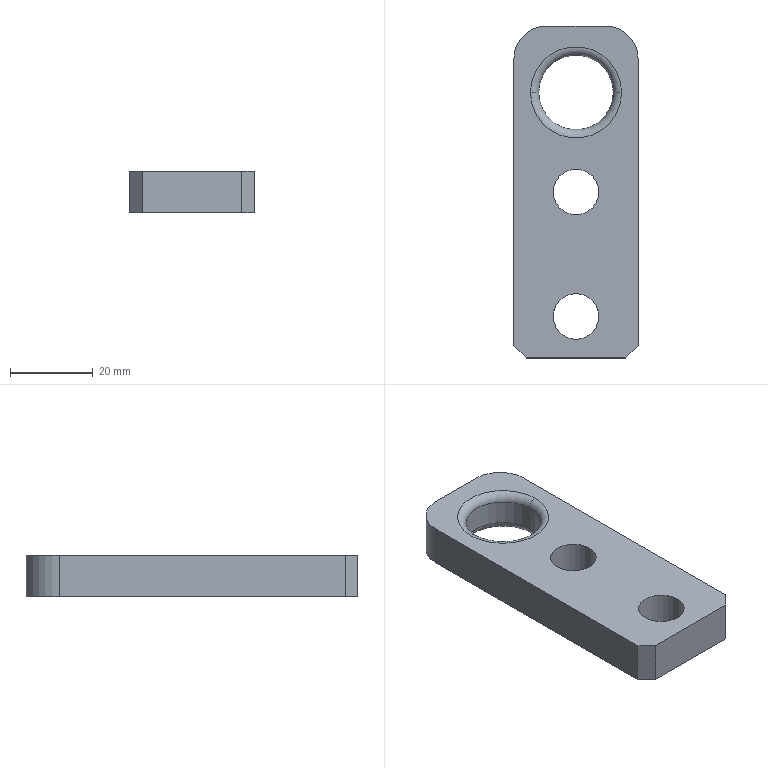Part | Creo | features DATUM PLANE 3, CHAMFER 1, COORDINATE SYSTEM 1, CURVE 1, PROTRUSION 1, ROUND 1 | 1 solid | 20 faces | box 30 x 80 x 10 mm | volume 19088 mm3 | plane 8 | cylinder 8 | torus 4 | commonest cylinder face diameters 11 x4 16 x2 18 x2
STEP:
#1=CARTESIAN_POINT('',(0.,0.,0.));
#2=DIRECTION('',(0.,0.,1.));
#3=DIRECTION('',(1.,0.,0.));
#4=AXIS2_PLACEMENT_3D('',#1,#2,#3);
#5=CARTESIAN_POINT('',(15.,-37.,0.));
#6=VERTEX_POINT('',#5);
#7=CARTESIAN_POINT('',(12.,-40.,0.));
#8=VERTEX_POINT('',#7);
#9=CARTESIAN_POINT('',(15.,-37.,0.));
#10=DIRECTION('',(-0.7071,-0.7071,0.));
#11=VECTOR('',#10,4.243);
#12=LINE('',#9,#11);
#13=EDGE_CURVE('',#6,#8,#12,.T.);
#14=ORIENTED_EDGE('',*,*,#13,.F.);
#15=CARTESIAN_POINT('',(15.,32.,0.));
#16=VERTEX_POINT('',#15);
#17=CARTESIAN_POINT('',(15.,-37.,0.));
#18=DIRECTION('',(0.,1.,0.));
#19=VECTOR('',#18,69.);
#20=LINE('',#17,#19);
#21=EDGE_CURVE('',#6,#16,#20,.T.);
#22=ORIENTED_EDGE('',*,*,#21,.T.);
#23=CARTESIAN_POINT('',(7.,40.,0.));
#24=VERTEX_POINT('',#23);
#25=CARTESIAN_POINT('',(7.,32.,0.));
#26=DIRECTION('',(0.,0.,1.));
#27=DIRECTION('',(1.,0.,0.));
#28=AXIS2_PLACEMENT_3D('',#25,#26,#27);
#29=CIRCLE('',#28,8.);
#30=EDGE_CURVE('',#16,#24,#29,.T.);
#31=ORIENTED_EDGE('',*,*,#30,.T.);
#32=CARTESIAN_POINT('',(-7.,40.,0.));
#33=VERTEX_POINT('',#32);
#34=CARTESIAN_POINT('',(7.,40.,0.));
#35=DIRECTION('',(-1.,0.,0.));
#36=VECTOR('',#35,14.);
#37=LINE('',#34,#36);
#38=EDGE_CURVE('',#24,#33,#37,.T.);
#39=ORIENTED_EDGE('',*,*,#38,.T.);
#40=CARTESIAN_POINT('',(-15.,32.,0.));
#41=VERTEX_POINT('',#40);
#42=CARTESIAN_POINT('',(-7.,32.,0.));
#43=DIRECTION('',(0.,0.,1.));
#44=DIRECTION('',(0.,1.,0.));
#45=AXIS2_PLACEMENT_3D('',#42,#43,#44);
#46=CIRCLE('',#45,8.);
#47=EDGE_CURVE('',#33,#41,#46,.T.);
#48=ORIENTED_EDGE('',*,*,#47,.T.);
#49=CARTESIAN_POINT('',(-15.,-37.,0.));
#50=VERTEX_POINT('',#49);
#51=CARTESIAN_POINT('',(-15.,32.,0.));
#52=DIRECTION('',(0.,-1.,0.));
#53=VECTOR('',#52,69.);
#54=LINE('',#51,#53);
#55=EDGE_CURVE('',#41,#50,#54,.T.);
#56=ORIENTED_EDGE('',*,*,#55,.T.);
#57=CARTESIAN_POINT('',(-12.,-40.,0.));
#58=VERTEX_POINT('',#57);
#59=CARTESIAN_POINT('',(-12.,-40.,0.));
#60=DIRECTION('',(-0.7071,0.7071,0.));
#61=VECTOR('',#60,4.243);
#62=LINE('',#59,#61);
#63=EDGE_CURVE('',#58,#50,#62,.T.);
#64=ORIENTED_EDGE('',*,*,#63,.F.);
#65=CARTESIAN_POINT('',(-12.,-40.,0.));
#66=DIRECTION('',(1.,0.,0.));
#67=VECTOR('',#66,24.);
#68=LINE('',#65,#67);
#69=EDGE_CURVE('',#58,#8,#68,.T.);
#70=ORIENTED_EDGE('',*,*,#69,.T.);
#71=EDGE_LOOP('',(#14,#22,#31,#39,#48,#56,#64,#70));
#72=FACE_OUTER_BOUND('',#71,.F.);
#73=CARTESIAN_POINT('',(5.5,0.,0.));
#74=VERTEX_POINT('',#73);
#75=CARTESIAN_POINT('',(-5.5,0.,0.));
#76=VERTEX_POINT('',#75);
#77=CARTESIAN_POINT('',(0.,0.,0.));
#78=DIRECTION('',(0.,0.,-1.));
#79=DIRECTION('',(1.,0.,0.));
#80=AXIS2_PLACEMENT_3D('',#77,#78,#79);
#81=CIRCLE('',#80,5.5);
#82=EDGE_CURVE('',#74,#76,#81,.T.);
#83=ORIENTED_EDGE('',*,*,#82,.T.);
#84=CARTESIAN_POINT('',(0.,0.,0.));
#85=DIRECTION('',(0.,0.,-1.));
#86=DIRECTION('',(-1.,0.,0.));
#87=AXIS2_PLACEMENT_3D('',#84,#85,#86);
#88=CIRCLE('',#87,5.5);
#89=EDGE_CURVE('',#76,#74,#88,.T.);
#90=ORIENTED_EDGE('',*,*,#89,.T.);
#91=EDGE_LOOP('',(#83,#90));
#92=FACE_BOUND('',#91,.F.);
#93=CARTESIAN_POINT('',(5.5,-30.,0.));
#94=VERTEX_POINT('',#93);
#95=CARTESIAN_POINT('',(-5.5,-30.,0.));
#96=VERTEX_POINT('',#95);
#97=CARTESIAN_POINT('',(0.,-30.,0.));
#98=DIRECTION('',(0.,0.,-1.));
#99=DIRECTION('',(1.,0.,0.));
#100=AXIS2_PLACEMENT_3D('',#97,#98,#99);
#101=CIRCLE('',#100,5.5);
#102=EDGE_CURVE('',#94,#96,#101,.T.);
#103=ORIENTED_EDGE('',*,*,#102,.T.);
#104=CARTESIAN_POINT('',(0.,-30.,0.));
#105=DIRECTION('',(0.,0.,-1.));
#106=DIRECTION('',(-1.,0.,0.));
#107=AXIS2_PLACEMENT_3D('',#104,#105,#106);
#108=CIRCLE('',#107,5.5);
#109=EDGE_CURVE('',#96,#94,#108,.T.);
#110=ORIENTED_EDGE('',*,*,#109,.T.);
#111=EDGE_LOOP('',(#103,#110));
#112=FACE_BOUND('',#111,.F.);
#113=CARTESIAN_POINT('',(-11.,24.,0.));
#114=VERTEX_POINT('',#113);
#115=CARTESIAN_POINT('',(11.,24.,0.));
#116=VERTEX_POINT('',#115);
#117=CARTESIAN_POINT('',(0.,24.,0.));
#118=DIRECTION('',(0.,0.,1.));
#119=DIRECTION('',(-1.,0.,0.));
#120=AXIS2_PLACEMENT_3D('',#117,#118,#119);
#121=CIRCLE('',#120,11.);
#122=EDGE_CURVE('',#114,#116,#121,.T.);
#123=ORIENTED_EDGE('',*,*,#122,.F.);
#124=CARTESIAN_POINT('',(0.,24.,0.));
#125=DIRECTION('',(0.,0.,1.));
#126=DIRECTION('',(1.,0.,0.));
#127=AXIS2_PLACEMENT_3D('',#124,#125,#126);
#128=CIRCLE('',#127,11.);
#129=EDGE_CURVE('',#116,#114,#128,.T.);
#130=ORIENTED_EDGE('',*,*,#129,.F.);
#131=EDGE_LOOP('',(#123,#130));
#132=FACE_BOUND('',#131,.F.);
#133=CARTESIAN_POINT('',(0.,0.,0.));
#134=DIRECTION('',(0.,0.,1.));
#135=DIRECTION('',(1.,0.,0.));
#136=AXIS2_PLACEMENT_3D('',#133,#134,#135);
#137=PLANE('',#136);
#138=ADVANCED_FACE('',(#72,#92,#112,#132),#137,.F.);
#139=ORIENTED_EDGE('',*,*,#102,.F.);
#140=CARTESIAN_POINT('',(5.5,-30.,10.));
#141=VERTEX_POINT('',#140);
#142=CARTESIAN_POINT('',(5.5,-30.,0.));
#143=DIRECTION('',(0.,0.,1.));
#144=VECTOR('',#143,10.);
#145=LINE('',#142,#144);
#146=EDGE_CURVE('',#94,#141,#145,.T.);
#147=ORIENTED_EDGE('',*,*,#146,.T.);
#148=CARTESIAN_POINT('',(-5.5,-30.,10.));
#149=VERTEX_POINT('',#148);
#150=CARTESIAN_POINT('',(0.,-30.,10.));
#151=DIRECTION('',(0.,0.,-1.));
#152=DIRECTION('',(1.,0.,0.));
#153=AXIS2_PLACEMENT_3D('',#150,#151,#152);
#154=CIRCLE('',#153,5.5);
#155=EDGE_CURVE('',#141,#149,#154,.T.);
#156=ORIENTED_EDGE('',*,*,#155,.T.);
#157=CARTESIAN_POINT('',(-5.5,-30.,0.));
#158=DIRECTION('',(0.,0.,1.));
#159=VECTOR('',#158,10.);
#160=LINE('',#157,#159);
#161=EDGE_CURVE('',#96,#149,#160,.T.);
#162=ORIENTED_EDGE('',*,*,#161,.F.);
#163=EDGE_LOOP('',(#139,#147,#156,#162));
#164=FACE_OUTER_BOUND('',#163,.F.);
#165=CARTESIAN_POINT('',(0.,-30.,0.));
#166=DIRECTION('',(0.,0.,1.));
#167=DIRECTION('',(1.,0.,0.));
#168=AXIS2_PLACEMENT_3D('',#165,#166,#167);
#169=CYLINDRICAL_SURFACE('',#168,5.5);
#170=ADVANCED_FACE('',(#164),#169,.F.);
#171=ORIENTED_EDGE('',*,*,#109,.F.);
#172=ORIENTED_EDGE('',*,*,#161,.T.);
#173=CARTESIAN_POINT('',(0.,-30.,10.));
#174=DIRECTION('',(0.,0.,-1.));
#175=DIRECTION('',(-1.,0.,0.));
#176=AXIS2_PLACEMENT_3D('',#173,#174,#175);
#177=CIRCLE('',#176,5.5);
#178=EDGE_CURVE('',#149,#141,#177,.T.);
#179=ORIENTED_EDGE('',*,*,#178,.T.);
#180=ORIENTED_EDGE('',*,*,#146,.F.);
#181=EDGE_LOOP('',(#171,#172,#179,#180));
#182=FACE_OUTER_BOUND('',#181,.F.);
#183=CARTESIAN_POINT('',(0.,-30.,0.));
#184=DIRECTION('',(0.,0.,1.));
#185=DIRECTION('',(1.,0.,0.));
#186=AXIS2_PLACEMENT_3D('',#183,#184,#185);
#187=CYLINDRICAL_SURFACE('',#186,5.5);
#188=ADVANCED_FACE('',(#182),#187,.F.);
#189=CARTESIAN_POINT('',(12.,-40.,10.));
#190=VERTEX_POINT('',#189);
#191=CARTESIAN_POINT('',(15.,-37.,10.));
#192=VERTEX_POINT('',#191);
#193=CARTESIAN_POINT('',(12.,-40.,10.));
#194=DIRECTION('',(0.7071,0.7071,0.));
#195=VECTOR('',#194,4.243);
#196=LINE('',#193,#195);
#197=EDGE_CURVE('',#190,#192,#196,.T.);
#198=ORIENTED_EDGE('',*,*,#197,.F.);
#199=CARTESIAN_POINT('',(-12.,-40.,10.));
#200=VERTEX_POINT('',#199);
#201=CARTESIAN_POINT('',(-12.,-40.,10.));
#202=DIRECTION('',(1.,0.,0.));
#203=VECTOR('',#202,24.);
#204=LINE('',#201,#203);
#205=EDGE_CURVE('',#200,#190,#204,.T.);
#206=ORIENTED_EDGE('',*,*,#205,.F.);
#207=CARTESIAN_POINT('',(-15.,-37.,10.));
#208=VERTEX_POINT('',#207);
#209=CARTESIAN_POINT('',(-15.,-37.,10.));
#210=DIRECTION('',(0.7071,-0.7071,0.));
#211=VECTOR('',#210,4.243);
#212=LINE('',#209,#211);
#213=EDGE_CURVE('',#208,#200,#212,.T.);
#214=ORIENTED_EDGE('',*,*,#213,.F.);
#215=CARTESIAN_POINT('',(-15.,32.,10.));
#216=VERTEX_POINT('',#215);
#217=CARTESIAN_POINT('',(-15.,32.,10.));
#218=DIRECTION('',(0.,-1.,0.));
#219=VECTOR('',#218,69.);
#220=LINE('',#217,#219);
#221=EDGE_CURVE('',#216,#208,#220,.T.);
#222=ORIENTED_EDGE('',*,*,#221,.F.);
#223=CARTESIAN_POINT('',(-7.,40.,10.));
#224=VERTEX_POINT('',#223);
#225=CARTESIAN_POINT('',(-7.,32.,10.));
#226=DIRECTION('',(0.,0.,1.));
#227=DIRECTION('',(0.,1.,0.));
#228=AXIS2_PLACEMENT_3D('',#225,#226,#227);
#229=CIRCLE('',#228,8.);
#230=EDGE_CURVE('',#224,#216,#229,.T.);
#231=ORIENTED_EDGE('',*,*,#230,.F.);
#232=CARTESIAN_POINT('',(7.,40.,10.));
#233=VERTEX_POINT('',#232);
#234=CARTESIAN_POINT('',(7.,40.,10.));
#235=DIRECTION('',(-1.,0.,0.));
#236=VECTOR('',#235,14.);
#237=LINE('',#234,#236);
#238=EDGE_CURVE('',#233,#224,#237,.T.);
#239=ORIENTED_EDGE('',*,*,#238,.F.);
#240=CARTESIAN_POINT('',(15.,32.,10.));
#241=VERTEX_POINT('',#240);
#242=CARTESIAN_POINT('',(7.,32.,10.));
#243=DIRECTION('',(0.,0.,1.));
#244=DIRECTION('',(1.,0.,0.));
#245=AXIS2_PLACEMENT_3D('',#242,#243,#244);
#246=CIRCLE('',#245,8.);
#247=EDGE_CURVE('',#241,#233,#246,.T.);
#248=ORIENTED_EDGE('',*,*,#247,.F.);
#249=CARTESIAN_POINT('',(15.,-37.,10.));
#250=DIRECTION('',(0.,1.,0.));
#251=VECTOR('',#250,69.);
#252=LINE('',#249,#251);
#253=EDGE_CURVE('',#192,#241,#252,.T.);
#254=ORIENTED_EDGE('',*,*,#253,.F.);
#255=EDGE_LOOP('',(#198,#206,#214,#222,#231,#239,#248,#254));
#256=FACE_OUTER_BOUND('',#255,.F.);
#257=CARTESIAN_POINT('',(5.5,0.,10.));
#258=VERTEX_POINT('',#257);
#259=CARTESIAN_POINT('',(-5.5,0.,10.));
#260=VERTEX_POINT('',#259);
#261=CARTESIAN_POINT('',(0.,0.,10.));
#262=DIRECTION('',(0.,0.,-1.));
#263=DIRECTION('',(1.,0.,0.));
#264=AXIS2_PLACEMENT_3D('',#261,#262,#263);
#265=CIRCLE('',#264,5.5);
#266=EDGE_CURVE('',#258,#260,#265,.T.);
#267=ORIENTED_EDGE('',*,*,#266,.F.);
#268=CARTESIAN_POINT('',(0.,0.,10.));
#269=DIRECTION('',(0.,0.,-1.));
#270=DIRECTION('',(-1.,0.,0.));
#271=AXIS2_PLACEMENT_3D('',#268,#269,#270);
#272=CIRCLE('',#271,5.5);
#273=EDGE_CURVE('',#260,#258,#272,.T.);
#274=ORIENTED_EDGE('',*,*,#273,.F.);
#275=EDGE_LOOP('',(#267,#274));
#276=FACE_BOUND('',#275,.F.);
#277=ORIENTED_EDGE('',*,*,#155,.F.);
#278=ORIENTED_EDGE('',*,*,#178,.F.);
#279=EDGE_LOOP('',(#277,#278));
#280=FACE_BOUND('',#279,.F.);
#281=CARTESIAN_POINT('',(11.,24.,10.));
#282=VERTEX_POINT('',#281);
#283=CARTESIAN_POINT('',(-11.,24.,10.));
#284=VERTEX_POINT('',#283);
#285=CARTESIAN_POINT('',(0.,24.,10.));
#286=DIRECTION('',(0.,0.,-1.));
#287=DIRECTION('',(1.,0.,0.));
#288=AXIS2_PLACEMENT_3D('',#285,#286,#287);
#289=CIRCLE('',#288,11.);
#290=EDGE_CURVE('',#282,#284,#289,.T.);
#291=ORIENTED_EDGE('',*,*,#290,.F.);
#292=CARTESIAN_POINT('',(0.,24.,10.));
#293=DIRECTION('',(0.,0.,-1.));
#294=DIRECTION('',(-1.,0.,0.));
#295=AXIS2_PLACEMENT_3D('',#292,#293,#294);
#296=CIRCLE('',#295,11.);
#297=EDGE_CURVE('',#284,#282,#296,.T.);
#298=ORIENTED_EDGE('',*,*,#297,.F.);
#299=EDGE_LOOP('',(#291,#298));
#300=FACE_BOUND('',#299,.F.);
#301=CARTESIAN_POINT('',(0.,0.,10.));
#302=DIRECTION('',(0.,0.,1.));
#303=DIRECTION('',(1.,0.,0.));
#304=AXIS2_PLACEMENT_3D('',#301,#302,#303);
#305=PLANE('',#304);
#306=ADVANCED_FACE('',(#256,#276,#280,#300),#305,.T.);
#307=ORIENTED_EDGE('',*,*,#82,.F.);
#308=CARTESIAN_POINT('',(5.5,0.,0.));
#309=DIRECTION('',(0.,0.,1.));
#310=VECTOR('',#309,10.);
#311=LINE('',#308,#310);
#312=EDGE_CURVE('',#74,#258,#311,.T.);
#313=ORIENTED_EDGE('',*,*,#312,.T.);
#314=ORIENTED_EDGE('',*,*,#266,.T.);
#315=CARTESIAN_POINT('',(-5.5,0.,0.));
#316=DIRECTION('',(0.,0.,1.));
#317=VECTOR('',#316,10.);
#318=LINE('',#315,#317);
#319=EDGE_CURVE('',#76,#260,#318,.T.);
#320=ORIENTED_EDGE('',*,*,#319,.F.);
#321=EDGE_LOOP('',(#307,#313,#314,#320));
#322=FACE_OUTER_BOUND('',#321,.F.);
#323=CARTESIAN_POINT('',(0.,0.,0.));
#324=DIRECTION('',(0.,0.,1.));
#325=DIRECTION('',(1.,0.,0.));
#326=AXIS2_PLACEMENT_3D('',#323,#324,#325);
#327=CYLINDRICAL_SURFACE('',#326,5.5);
#328=ADVANCED_FACE('',(#322),#327,.F.);
#329=ORIENTED_EDGE('',*,*,#89,.F.);
#330=ORIENTED_EDGE('',*,*,#319,.T.);
#331=ORIENTED_EDGE('',*,*,#273,.T.);
#332=ORIENTED_EDGE('',*,*,#312,.F.);
#333=EDGE_LOOP('',(#329,#330,#331,#332));
#334=FACE_OUTER_BOUND('',#333,.F.);
#335=CARTESIAN_POINT('',(0.,0.,0.));
#336=DIRECTION('',(0.,0.,1.));
#337=DIRECTION('',(1.,0.,0.));
#338=AXIS2_PLACEMENT_3D('',#335,#336,#337);
#339=CYLINDRICAL_SURFACE('',#338,5.5);
#340=ADVANCED_FACE('',(#334),#339,.F.);
#341=ORIENTED_EDGE('',*,*,#13,.T.);
#342=CARTESIAN_POINT('',(12.,-40.,10.));
#343=DIRECTION('',(0.,0.,-1.));
#344=VECTOR('',#343,10.);
#345=LINE('',#342,#344);
#346=EDGE_CURVE('',#190,#8,#345,.T.);
#347=ORIENTED_EDGE('',*,*,#346,.F.);
#348=ORIENTED_EDGE('',*,*,#197,.T.);
#349=CARTESIAN_POINT('',(15.,-37.,10.));
#350=DIRECTION('',(0.,0.,-1.));
#351=VECTOR('',#350,10.);
#352=LINE('',#349,#351);
#353=EDGE_CURVE('',#192,#6,#352,.T.);
#354=ORIENTED_EDGE('',*,*,#353,.T.);
#355=EDGE_LOOP('',(#341,#347,#348,#354));
#356=FACE_OUTER_BOUND('',#355,.F.);
#357=CARTESIAN_POINT('',(13.5,-38.5,5.));
#358=DIRECTION('',(0.7071,-0.7071,0.));
#359=DIRECTION('',(-0.7071,-0.7071,0.));
#360=AXIS2_PLACEMENT_3D('',#357,#358,#359);
#361=PLANE('',#360);
#362=ADVANCED_FACE('',(#356),#361,.T.);
#363=ORIENTED_EDGE('',*,*,#346,.T.);
#364=ORIENTED_EDGE('',*,*,#69,.F.);
#365=CARTESIAN_POINT('',(-12.,-40.,10.));
#366=DIRECTION('',(0.,0.,-1.));
#367=VECTOR('',#366,10.);
#368=LINE('',#365,#367);
#369=EDGE_CURVE('',#200,#58,#368,.T.);
#370=ORIENTED_EDGE('',*,*,#369,.F.);
#371=ORIENTED_EDGE('',*,*,#205,.T.);
#372=EDGE_LOOP('',(#363,#364,#370,#371));
#373=FACE_OUTER_BOUND('',#372,.F.);
#374=CARTESIAN_POINT('',(-15.,-40.,0.));
#375=DIRECTION('',(0.,-1.,0.));
#376=DIRECTION('',(1.,0.,0.));
#377=AXIS2_PLACEMENT_3D('',#374,#375,#376);
#378=PLANE('',#377);
#379=ADVANCED_FACE('',(#373),#378,.T.);
#380=ORIENTED_EDGE('',*,*,#63,.T.);
#381=CARTESIAN_POINT('',(-15.,-37.,10.));
#382=DIRECTION('',(0.,0.,-1.));
#383=VECTOR('',#382,10.);
#384=LINE('',#381,#383);
#385=EDGE_CURVE('',#208,#50,#384,.T.);
#386=ORIENTED_EDGE('',*,*,#385,.F.);
#387=ORIENTED_EDGE('',*,*,#213,.T.);
#388=ORIENTED_EDGE('',*,*,#369,.T.);
#389=EDGE_LOOP('',(#380,#386,#387,#388));
#390=FACE_OUTER_BOUND('',#389,.F.);
#391=CARTESIAN_POINT('',(-13.5,-38.5,5.));
#392=DIRECTION('',(-0.7071,-0.7071,0.));
#393=DIRECTION('',(-0.7071,0.7071,0.));
#394=AXIS2_PLACEMENT_3D('',#391,#392,#393);
#395=PLANE('',#394);
#396=ADVANCED_FACE('',(#390),#395,.T.);
#397=ORIENTED_EDGE('',*,*,#385,.T.);
#398=ORIENTED_EDGE('',*,*,#55,.F.);
#399=CARTESIAN_POINT('',(-15.,32.,0.));
#400=DIRECTION('',(0.,0.,1.));
#401=VECTOR('',#400,10.);
#402=LINE('',#399,#401);
#403=EDGE_CURVE('',#41,#216,#402,.T.);
#404=ORIENTED_EDGE('',*,*,#403,.T.);
#405=ORIENTED_EDGE('',*,*,#221,.T.);
#406=EDGE_LOOP('',(#397,#398,#404,#405));
#407=FACE_OUTER_BOUND('',#406,.F.);
#408=CARTESIAN_POINT('',(-15.,32.,0.));
#409=DIRECTION('',(-1.,0.,0.));
#410=DIRECTION('',(0.,-1.,0.));
#411=AXIS2_PLACEMENT_3D('',#408,#409,#410);
#412=PLANE('',#411);
#413=ADVANCED_FACE('',(#407),#412,.T.);
#414=ORIENTED_EDGE('',*,*,#47,.F.);
#415=CARTESIAN_POINT('',(-7.,40.,0.));
#416=DIRECTION('',(0.,0.,1.));
#417=VECTOR('',#416,10.);
#418=LINE('',#415,#417);
#419=EDGE_CURVE('',#33,#224,#418,.T.);
#420=ORIENTED_EDGE('',*,*,#419,.T.);
#421=ORIENTED_EDGE('',*,*,#230,.T.);
#422=ORIENTED_EDGE('',*,*,#403,.F.);
#423=EDGE_LOOP('',(#414,#420,#421,#422));
#424=FACE_OUTER_BOUND('',#423,.F.);
#425=CARTESIAN_POINT('',(-7.,32.,0.));
#426=DIRECTION('',(0.,0.,1.));
#427=DIRECTION('',(1.,0.,0.));
#428=AXIS2_PLACEMENT_3D('',#425,#426,#427);
#429=CYLINDRICAL_SURFACE('',#428,8.);
#430=ADVANCED_FACE('',(#424),#429,.T.);
#431=ORIENTED_EDGE('',*,*,#38,.F.);
#432=CARTESIAN_POINT('',(7.,40.,0.));
#433=DIRECTION('',(0.,0.,1.));
#434=VECTOR('',#433,10.);
#435=LINE('',#432,#434);
#436=EDGE_CURVE('',#24,#233,#435,.T.);
#437=ORIENTED_EDGE('',*,*,#436,.T.);
#438=ORIENTED_EDGE('',*,*,#238,.T.);
#439=ORIENTED_EDGE('',*,*,#419,.F.);
#440=EDGE_LOOP('',(#431,#437,#438,#439));
#441=FACE_OUTER_BOUND('',#440,.F.);
#442=CARTESIAN_POINT('',(7.,40.,0.));
#443=DIRECTION('',(0.,1.,0.));
#444=DIRECTION('',(-1.,0.,0.));
#445=AXIS2_PLACEMENT_3D('',#442,#443,#444);
#446=PLANE('',#445);
#447=ADVANCED_FACE('',(#441),#446,.T.);
#448=ORIENTED_EDGE('',*,*,#30,.F.);
#449=CARTESIAN_POINT('',(15.,32.,0.));
#450=DIRECTION('',(0.,0.,1.));
#451=VECTOR('',#450,10.);
#452=LINE('',#449,#451);
#453=EDGE_CURVE('',#16,#241,#452,.T.);
#454=ORIENTED_EDGE('',*,*,#453,.T.);
#455=ORIENTED_EDGE('',*,*,#247,.T.);
#456=ORIENTED_EDGE('',*,*,#436,.F.);
#457=EDGE_LOOP('',(#448,#454,#455,#456));
#458=FACE_OUTER_BOUND('',#457,.F.);
#459=CARTESIAN_POINT('',(7.,32.,0.));
#460=DIRECTION('',(0.,0.,1.));
#461=DIRECTION('',(1.,0.,0.));
#462=AXIS2_PLACEMENT_3D('',#459,#460,#461);
#463=CYLINDRICAL_SURFACE('',#462,8.);
#464=ADVANCED_FACE('',(#458),#463,.T.);
#465=ORIENTED_EDGE('',*,*,#353,.F.);
#466=ORIENTED_EDGE('',*,*,#253,.T.);
#467=ORIENTED_EDGE('',*,*,#453,.F.);
#468=ORIENTED_EDGE('',*,*,#21,.F.);
#469=EDGE_LOOP('',(#465,#466,#467,#468));
#470=FACE_OUTER_BOUND('',#469,.F.);
#471=CARTESIAN_POINT('',(15.,-40.,0.));
#472=DIRECTION('',(1.,0.,0.));
#473=DIRECTION('',(0.,1.,0.));
#474=AXIS2_PLACEMENT_3D('',#471,#472,#473);
#475=PLANE('',#474);
#476=ADVANCED_FACE('',(#470),#475,.T.);
#477=ORIENTED_EDGE('',*,*,#290,.T.);
#478=CARTESIAN_POINT('',(-9.,24.,8.));
#479=VERTEX_POINT('',#478);
#480=CARTESIAN_POINT('',(-11.,24.,8.));
#481=DIRECTION('',(0.,1.,0.));
#482=DIRECTION('',(0.,0.,1.));
#483=AXIS2_PLACEMENT_3D('',#480,#481,#482);
#484=CIRCLE('',#483,2.);
#485=EDGE_CURVE('',#284,#479,#484,.T.);
#486=ORIENTED_EDGE('',*,*,#485,.T.);
#487=CARTESIAN_POINT('',(9.,24.,8.));
#488=VERTEX_POINT('',#487);
#489=CARTESIAN_POINT('',(0.,24.,8.));
#490=DIRECTION('',(0.,0.,-1.));
#491=DIRECTION('',(1.,0.,0.));
#492=AXIS2_PLACEMENT_3D('',#489,#490,#491);
#493=CIRCLE('',#492,9.);
#494=EDGE_CURVE('',#488,#479,#493,.T.);
#495=ORIENTED_EDGE('',*,*,#494,.F.);
#496=CARTESIAN_POINT('',(11.,24.,8.));
#497=DIRECTION('',(0.,-1.,0.));
#498=DIRECTION('',(0.,0.,1.));
#499=AXIS2_PLACEMENT_3D('',#496,#497,#498);
#500=CIRCLE('',#499,2.);
#501=EDGE_CURVE('',#282,#488,#500,.T.);
#502=ORIENTED_EDGE('',*,*,#501,.F.);
#503=EDGE_LOOP('',(#477,#486,#495,#502));
#504=FACE_OUTER_BOUND('',#503,.F.);
#505=CARTESIAN_POINT('',(0.,24.,8.));
#506=DIRECTION('',(0.,0.,1.));
#507=DIRECTION('',(0.9998,0.02088,0.));
#508=AXIS2_PLACEMENT_3D('',#505,#506,#507);
#509=TOROIDAL_SURFACE('',#508,11.,2.);
#510=ADVANCED_FACE('',(#504),#509,.T.);
#511=ORIENTED_EDGE('',*,*,#297,.T.);
#512=ORIENTED_EDGE('',*,*,#501,.T.);
#513=CARTESIAN_POINT('',(0.,24.,8.));
#514=DIRECTION('',(0.,0.,-1.));
#515=DIRECTION('',(-1.,0.,0.));
#516=AXIS2_PLACEMENT_3D('',#513,#514,#515);
#517=CIRCLE('',#516,9.);
#518=EDGE_CURVE('',#479,#488,#517,.T.);
#519=ORIENTED_EDGE('',*,*,#518,.F.);
#520=ORIENTED_EDGE('',*,*,#485,.F.);
#521=EDGE_LOOP('',(#511,#512,#519,#520));
#522=FACE_OUTER_BOUND('',#521,.F.);
#523=CARTESIAN_POINT('',(0.,24.,8.));
#524=DIRECTION('',(0.,0.,1.));
#525=DIRECTION('',(-0.9998,-0.02088,0.));
#526=AXIS2_PLACEMENT_3D('',#523,#524,#525);
#527=TOROIDAL_SURFACE('',#526,11.,2.);
#528=ADVANCED_FACE('',(#522),#527,.T.);
#529=ORIENTED_EDGE('',*,*,#518,.T.);
#530=CARTESIAN_POINT('',(9.,24.,2.));
#531=VERTEX_POINT('',#530);
#532=CARTESIAN_POINT('',(9.,24.,2.));
#533=DIRECTION('',(0.,0.,1.));
#534=VECTOR('',#533,6.);
#535=LINE('',#532,#534);
#536=EDGE_CURVE('',#531,#488,#535,.T.);
#537=ORIENTED_EDGE('',*,*,#536,.F.);
#538=CARTESIAN_POINT('',(-9.,24.,2.));
#539=VERTEX_POINT('',#538);
#540=CARTESIAN_POINT('',(0.,24.,2.));
#541=DIRECTION('',(0.,0.,1.));
#542=DIRECTION('',(1.,0.,0.));
#543=AXIS2_PLACEMENT_3D('',#540,#541,#542);
#544=CIRCLE('',#543,9.);
#545=EDGE_CURVE('',#531,#539,#544,.T.);
#546=ORIENTED_EDGE('',*,*,#545,.T.);
#547=CARTESIAN_POINT('',(-9.,24.,2.));
#548=DIRECTION('',(0.,0.,1.));
#549=VECTOR('',#548,6.);
#550=LINE('',#547,#549);
#551=EDGE_CURVE('',#539,#479,#550,.T.);
#552=ORIENTED_EDGE('',*,*,#551,.T.);
#553=EDGE_LOOP('',(#529,#537,#546,#552));
#554=FACE_OUTER_BOUND('',#553,.F.);
#555=CARTESIAN_POINT('',(0.,24.,0.));
#556=DIRECTION('',(0.,0.,1.));
#557=DIRECTION('',(1.,0.,0.));
#558=AXIS2_PLACEMENT_3D('',#555,#556,#557);
#559=CYLINDRICAL_SURFACE('',#558,9.);
#560=ADVANCED_FACE('',(#554),#559,.F.);
#561=ORIENTED_EDGE('',*,*,#494,.T.);
#562=ORIENTED_EDGE('',*,*,#551,.F.);
#563=CARTESIAN_POINT('',(0.,24.,2.));
#564=DIRECTION('',(0.,0.,1.));
#565=DIRECTION('',(-1.,0.,0.));
#566=AXIS2_PLACEMENT_3D('',#563,#564,#565);
#567=CIRCLE('',#566,9.);
#568=EDGE_CURVE('',#539,#531,#567,.T.);
#569=ORIENTED_EDGE('',*,*,#568,.T.);
#570=ORIENTED_EDGE('',*,*,#536,.T.);
#571=EDGE_LOOP('',(#561,#562,#569,#570));
#572=FACE_OUTER_BOUND('',#571,.F.);
#573=CARTESIAN_POINT('',(0.,24.,0.));
#574=DIRECTION('',(0.,0.,1.));
#575=DIRECTION('',(1.,0.,0.));
#576=AXIS2_PLACEMENT_3D('',#573,#574,#575);
#577=CYLINDRICAL_SURFACE('',#576,9.);
#578=ADVANCED_FACE('',(#572),#577,.F.);
#579=ORIENTED_EDGE('',*,*,#122,.T.);
#580=CARTESIAN_POINT('',(11.,24.,2.));
#581=DIRECTION('',(0.,1.,0.));
#582=DIRECTION('',(0.,0.,-1.));
#583=AXIS2_PLACEMENT_3D('',#580,#581,#582);
#584=CIRCLE('',#583,2.);
#585=EDGE_CURVE('',#116,#531,#584,.T.);
#586=ORIENTED_EDGE('',*,*,#585,.T.);
#587=ORIENTED_EDGE('',*,*,#568,.F.);
#588=CARTESIAN_POINT('',(-11.,24.,2.));
#589=DIRECTION('',(0.,-1.,0.));
#590=DIRECTION('',(0.,0.,-1.));
#591=AXIS2_PLACEMENT_3D('',#588,#589,#590);
#592=CIRCLE('',#591,2.);
#593=EDGE_CURVE('',#114,#539,#592,.T.);
#594=ORIENTED_EDGE('',*,*,#593,.F.);
#595=EDGE_LOOP('',(#579,#586,#587,#594));
#596=FACE_OUTER_BOUND('',#595,.F.);
#597=CARTESIAN_POINT('',(0.,24.,2.));
#598=DIRECTION('',(0.,0.,1.));
#599=DIRECTION('',(-0.9999,0.0147,0.));
#600=AXIS2_PLACEMENT_3D('',#597,#598,#599);
#601=TOROIDAL_SURFACE('',#600,11.,2.);
#602=ADVANCED_FACE('',(#596),#601,.T.);
#603=ORIENTED_EDGE('',*,*,#129,.T.);
#604=ORIENTED_EDGE('',*,*,#593,.T.);
#605=ORIENTED_EDGE('',*,*,#545,.F.);
#606=ORIENTED_EDGE('',*,*,#585,.F.);
#607=EDGE_LOOP('',(#603,#604,#605,#606));
#608=FACE_OUTER_BOUND('',#607,.F.);
#609=CARTESIAN_POINT('',(0.,24.,2.));
#610=DIRECTION('',(0.,0.,1.));
#611=DIRECTION('',(0.9999,-0.0147,0.));
#612=AXIS2_PLACEMENT_3D('',#609,#610,#611);
#613=TOROIDAL_SURFACE('',#612,11.,2.);
#614=ADVANCED_FACE('',(#608),#613,.T.);
#615=CLOSED_SHELL('',(#138,#170,#188,#306,#328,#340,#362,#379,#396,#413,#430,#447,#464,#476,#510,#528,#560,#578,#602,#614));
#616=MANIFOLD_SOLID_BREP('',#615);
#617=(LENGTH_UNIT()NAMED_UNIT(*)SI_UNIT(.MILLI.,.METRE.));
#618=UNCERTAINTY_MEASURE_WITH_UNIT(LENGTH_MEASURE(0.008602),#617,'','');
#619=(NAMED_UNIT(*)PLANE_ANGLE_UNIT()SI_UNIT($,.RADIAN.));
#620=PLANE_ANGLE_MEASURE_WITH_UNIT(PLANE_ANGLE_MEASURE(0.01745),#619);
#621=(CONVERSION_BASED_UNIT('DEGREE',#620)NAMED_UNIT(*)PLANE_ANGLE_UNIT());
#622=(NAMED_UNIT(*)SI_UNIT($,.STERADIAN.)SOLID_ANGLE_UNIT());
#623=(GEOMETRIC_REPRESENTATION_CONTEXT(3)GLOBAL_UNCERTAINTY_ASSIGNED_CONTEXT((#618))GLOBAL_UNIT_ASSIGNED_CONTEXT((#617,#621,#622))REPRESENTATION_CONTEXT('',''));
#624=ADVANCED_BREP_SHAPE_REPRESENTATION('',(#4,#616),#623);